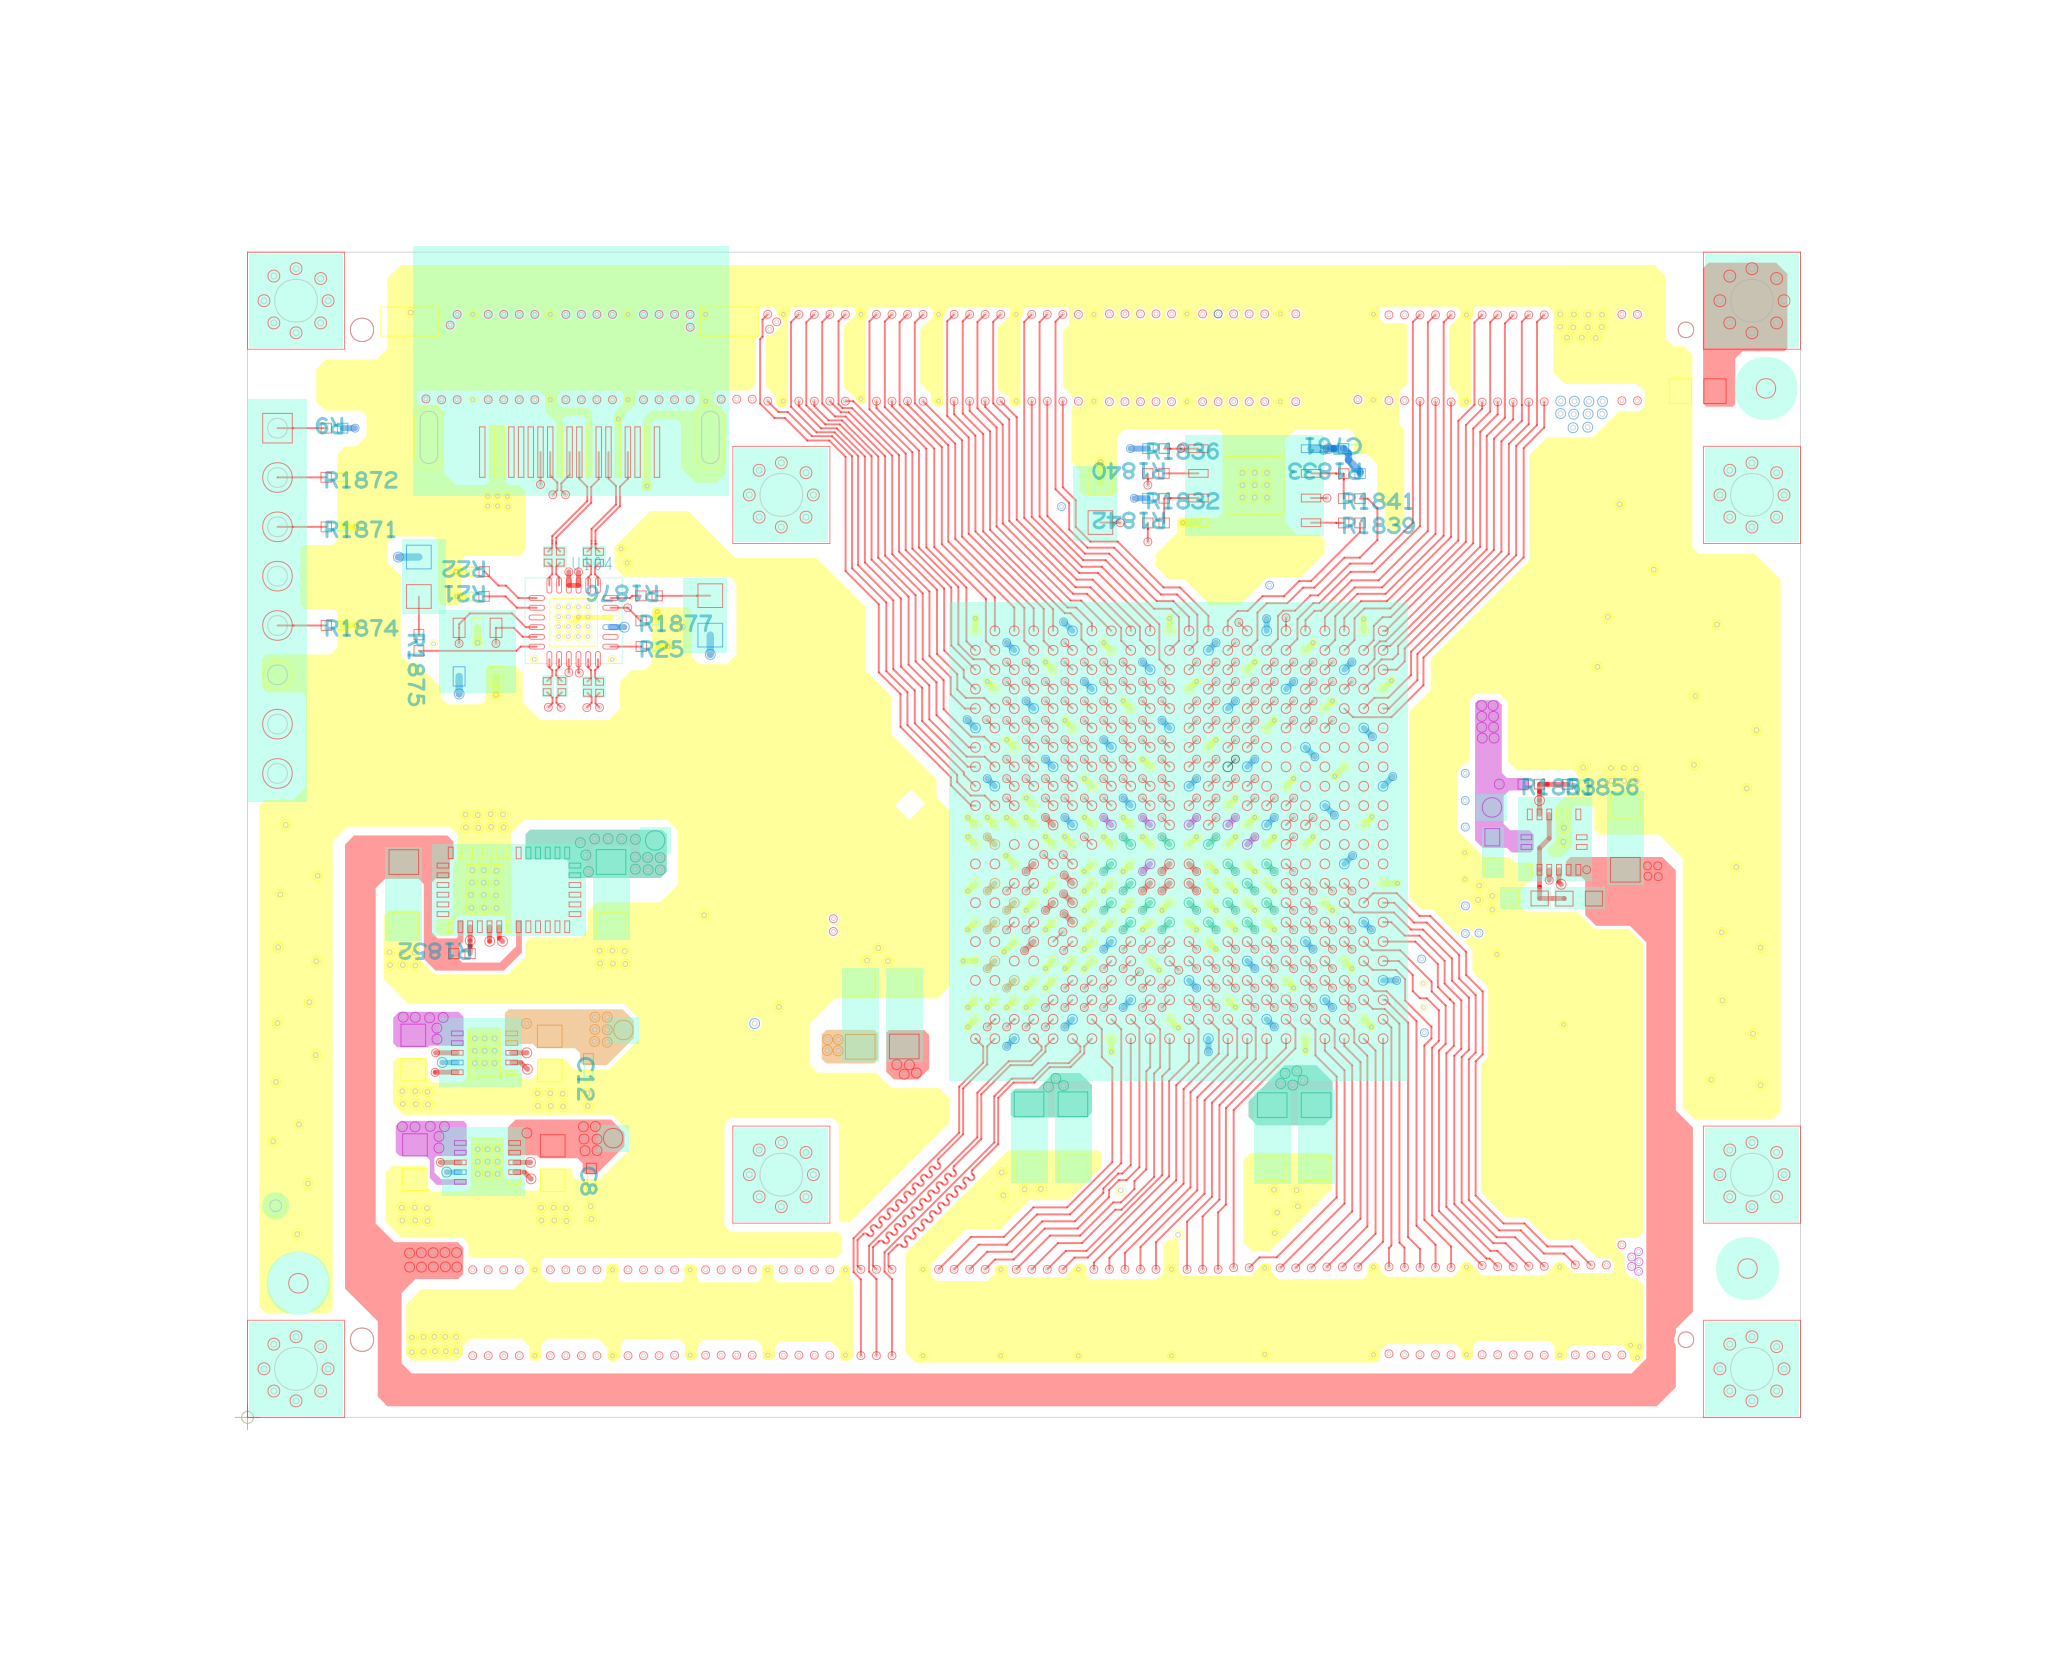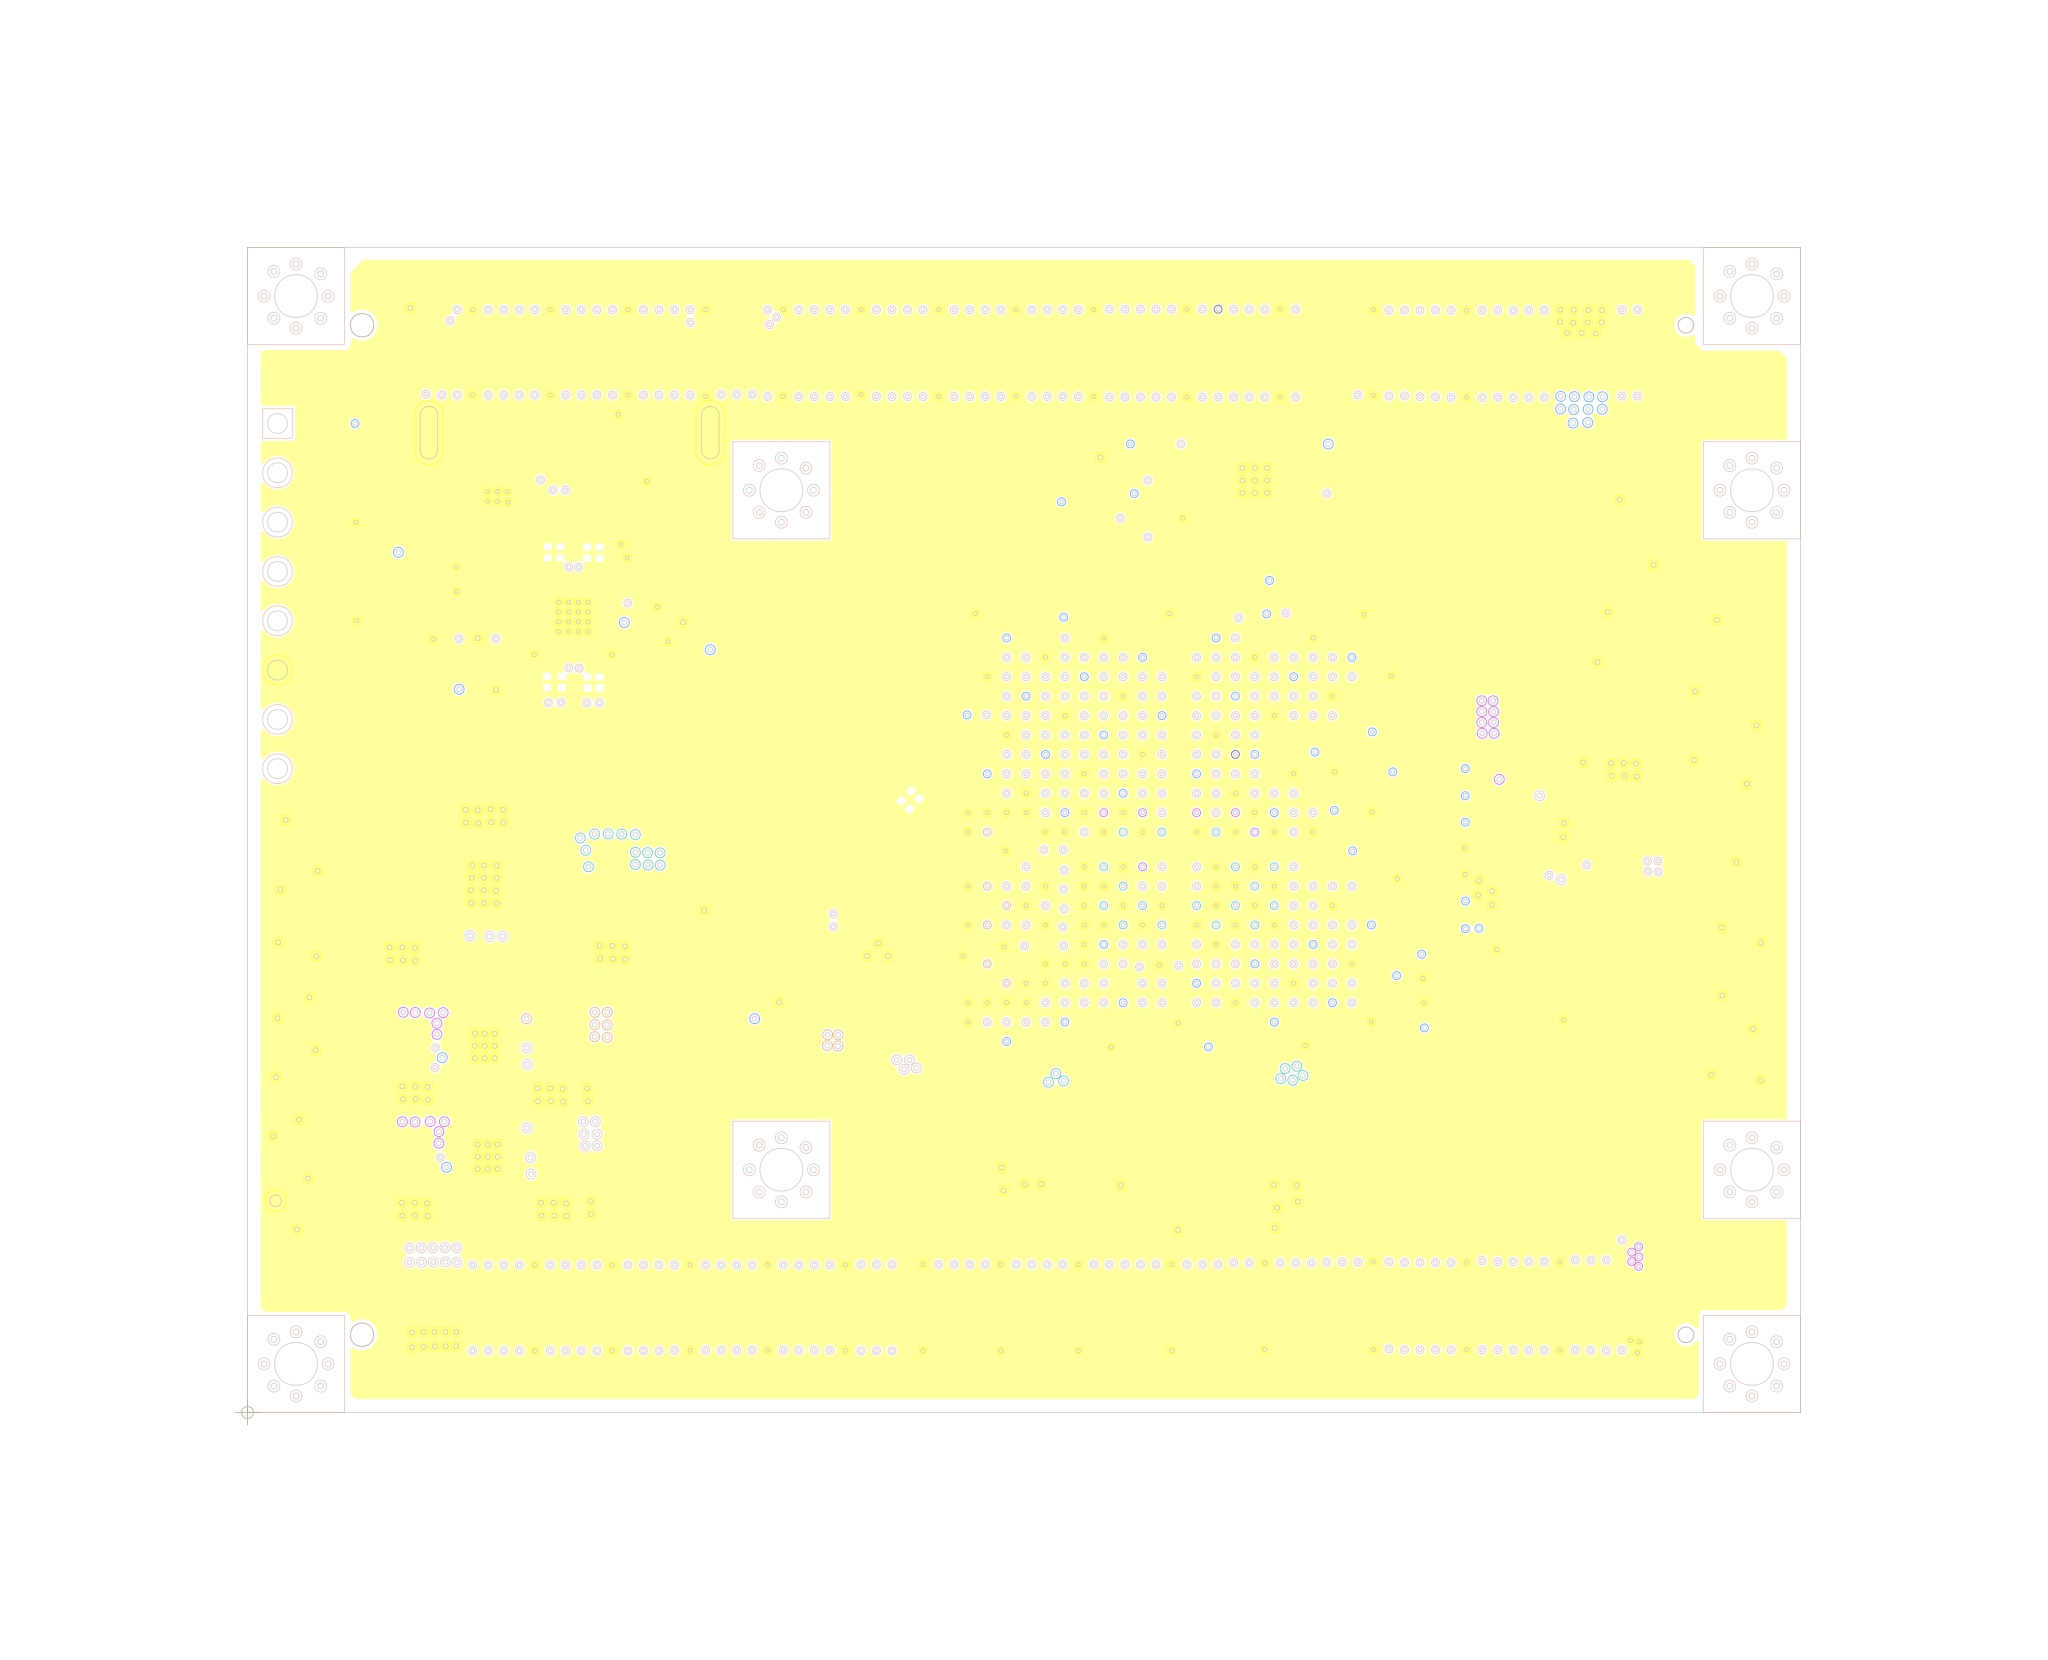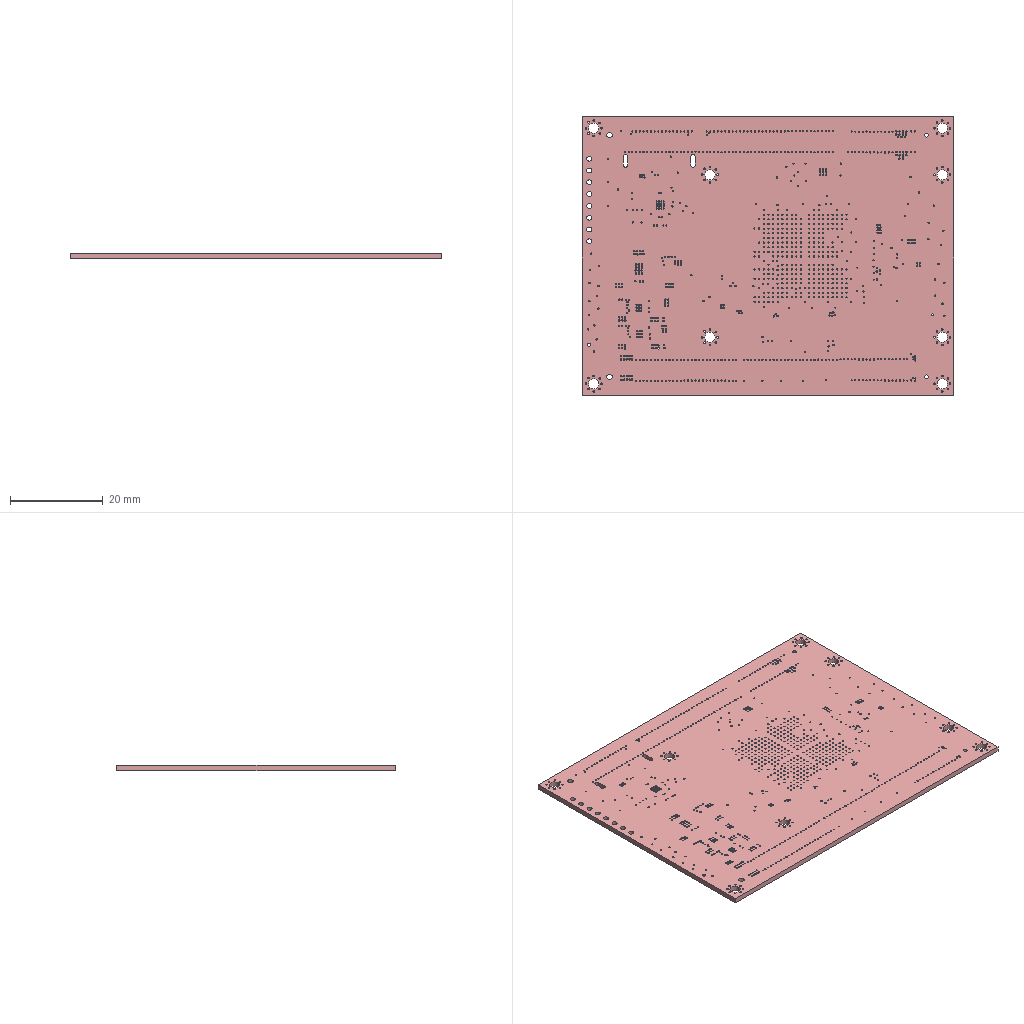Circuit board layout | Cadence Allegro | box 80 x 60 x 1.1 mm
Layer stack:
# Cadence Allegro layer stack of  (unit mm; from the constraint file cross-section; dielectric type: 0 not recorded (Allegro does not mark core vs prepreg), 3 surface material)
index,name,kind,layer,copper_thickness_mm,dielectric_type,dielectric_thickness_mm,dielectric_material,dielectric_constant
0,Top Surface,other,,,,,,
1,TOP,copper,TOP,0.0305,,,,
2,Dielectric1,dielectric,,,0,0.2032,FR-4,4.5
3,GND2,copper,GND2,0.0305,,,,
4,Dielectric2,dielectric,,,0,0.2032,FR-4,4.5
5,SIG3,copper,SIG3,0.0305,,,,
6,Dielectric3,dielectric,,,0,0.2032,FR-4,4.5
7,SIG4,copper,SIG4,0.0305,,,,
8,Dielectric4,dielectric,,,0,0.2032,FR-4,4.5
9,POWER5,copper,POWER5,0.0305,,,,
10,Dielectric5,dielectric,,,0,0.2032,FR-4,4.5
11,BOTTOM,copper,BOTTOM,0.0305,,,,
12,Bottom Surface,other,,,,,,
# drill layer pairs: low layer,high layer
drill_pair,TOP,BOTTOM
Part placement:
REFDES,COMP_VALUE,SYM_NAME,SYM_X,SYM_Y,SYM_ROTATE,SYM_MIRROR
C1,0.47uF/6.3V/10%/X5R/C0201,0201,1815.268,1086.576,180.000,YES
C2,0.47uF/6.3V/10%/X5R/C0201,0201,1815.260,1047.565,180.000,YES
C3,0.1uF/25V/10%/X5R/C0201,0201,1354.244,1251.889,135.000,YES
C4,0.1uF/25V/10%/X5R/C0201,0201,1334.672,1231.394,135.000,YES
C5,10uF/6.3V/10%/X5R/C0805,0805,339.614,517.452,270.000,NO
C6,0.1uF/50V/10%/X7R/C0402,0402,431.307,513.971,270.000,YES
C7,270P/6.3V/20%/X5R/C0402,0402,618.658,483.605,180.000,YES
C8,0.1uF/50V/10%/X7R/C0402,0402,697.516,488.137,270.000,NO
C9,47uF/6.3V/20%/X5R/C0805,0805,619.107,515.507,270.000,NO
C10,0.1uF/50V/10%/X7R/C0402,0402,425.205,736.184,270.000,YES
C11,47uF/6.3V/20%/X5R/C0805,0805,613.004,737.719,270.000,NO
C12,0.1uF/50V/10%/X7R/C0402,0402,691.414,710.349,270.000,NO
C13,10uF/6.3V/10%/X5R/C0805,0805,336.197,739.664,270.000,NO
C14,270P/6.3V/20%/X5R/C0402,0402,612.555,705.818,180.000,YES
C66,0.1uF/25V/10%/X5R/C0201,0201,2553.761,841.768,180.000,YES
C67,0.1uF/25V/10%/X5R/C0201,0201,2553.608,877.076,180.000,YES
C761,0.1uF/50V/10%/X7R/C0402,0402,2239.425,1964.287,180.000,NO
C763,100uF/6.3V/20%/X5R/C1206,T_1206,1773.209,569.491,90.000,YES
C764,4.7uF/6.3V/20%/X5R/C0402,0402,1887.404,1430.555,270.000,YES
C765,4.7uF/6.3V/20%/X5R/C0402,0402,2236.186,1189.759,180.000,YES
C766,100uF/6.3V/20%/X5R/C1206,T_1206,1585.041,570.750,270.000,NO
C767,100uF/6.3V/20%/X5R/C1206,T_1206,2119.165,569.587,90.000,YES
C768,100uF/6.3V/20%/X5R/C1206,T_1206,1673.984,570.757,270.000,NO
C769,0.47uF/6.3V/10%/X5R/C0201,0201,1925.198,1047.843,180.000,YES
C770,0.47uF/6.3V/10%/X5R/C0201,0201,2062.668,987.705,270.000,YES
C771,0.47uF/6.3V/10%/X5R/C0201,0201,1736.834,929.305,0.000,YES
C772,0.47uF/6.3V/10%/X5R/C0201,0201,1889.278,885.073,0.000,YES
C773,0.47uF/6.3V/10%/X5R/C0201,0201,1775.691,1236.027,180.000,YES
C774,0.47uF/6.3V/10%/X5R/C0201,0201,1559.332,791.280,270.000,YES
C775,0.47uF/6.3V/10%/X5R/C0201,0201,1983.760,989.024,270.000,YES
C776,0.47uF/6.3V/10%/X5R/C0201,0201,2101.346,1104.985,90.000,YES
C777,0.47uF/6.3V/10%/X5R/C0201,0201,2023.330,1028.285,90.000,YES
C778,0.47uF/6.3V/10%/X5R/C0201,0201,1756.062,1067.612,90.000,YES
C779,100uF/6.3V/20%/X5R/C1206,T_1206,1331.994,815.845,90.000,NO
C780,4.7uF/6.3V/20%/X5R/C0402,0402,1576.705,907.539,135.000,YES
C781,0.47uF/6.3V/10%/X5R/C0201,0201,1597.403,1008.921,0.000,YES
C782,100uF/6.3V/20%/X5R/C1206,T_1206,1379.805,1504.170,270.000,YES
C783,4.7uF/6.3V/20%/X5R/C0402,0402,1889.664,1311.894,270.000,YES
C784,4.7uF/6.3V/20%/X5R/C0402,0402,2264.650,1572.043,270.000,YES
C785,100uF/6.3V/20%/X5R/C1206,T_1206,2431.893,1489.047,270.000,YES
C786,4.7uF/6.3V/20%/X5R/C0402,0402,1890.236,1206.849,90.000,YES
C787,0.47uF/6.3V/10%/X5R/C0201,0201,2023.094,1215.693,90.000,YES
C788,0.47uF/6.3V/10%/X5R/C0201,0201,2063.562,1154.163,180.000,YES
C789,0.47uF/6.3V/10%/X5R/C0201,0201,1677.735,1215.385,90.000,YES
C790,0.47uF/6.3V/10%/X5R/C0201,0201,2102.239,1215.741,90.000,YES
C791,0.47uF/6.3V/10%/X5R/C0201,0201,1983.995,1413.098,90.000,YES
C792,0.47uF/6.3V/10%/X5R/C0201,0201,1776.037,1354.228,180.000,YES
C793,100uF/6.3V/20%/X5R/C1206,T_1206,1242.639,815.169,90.000,NO
C794,4.7uF/6.3V/20%/X5R/C0402,0402,1489.472,1027.803,0.000,YES
C795,0.47uF/6.3V/10%/X5R/C0201,0201,1483.481,934.388,0.000,YES
C796,100uF/6.3V/20%/X5R/C1206,T_1206,2167.176,569.035,270.000,NO
C797,4.7uF/6.3V/20%/X5R/C0402,0402,1887.876,983.961,90.000,YES
C798,100uF/6.3V/20%/X5R/C1206,T_1206,2078.175,569.035,270.000,NO
C799,4.7uF/6.3V/20%/X5R/C0402,0402,1757.832,1143.819,0.000,YES
C800,100uF/6.3V/20%/X5R/C1206,T_1206,2276.161,1387.556,270.000,YES
C801,4.7uF/6.3V/20%/X5R/C0402,0402,2083.622,1363.955,270.000,YES
C802,4.7uF/6.3V/20%/X5R/C0402,0402,2253.888,1026.907,0.000,YES
C803,0.47uF/6.3V/10%/X5R/C0201,0201,1795.243,988.367,90.000,YES
C804,0.47uF/6.3V/10%/X5R/C0201,0201,1716.691,1027.863,90.000,YES
C805,0.47uF/6.3V/10%/X5R/C0201,0201,1983.080,1153.632,180.000,YES
C806,0.47uF/6.3V/10%/X5R/C0201,0201,1834.935,1150.180,0.000,YES
C807,0.47uF/6.3V/10%/X5R/C0201,0201,2062.603,1066.526,270.000,YES
C808,0.47uF/6.3V/10%/X5R/C0201,0201,2229.205,801.348,180.000,YES
C809,0.47uF/6.3V/10%/X5R/C0201,0201,1795.599,1490.563,90.000,YES
C810,0.47uF/6.3V/10%/X5R/C0201,0201,1638.059,1373.665,270.000,YES
C811,0.47uF/6.3V/10%/X5R/C0201,0201,2003.454,929.020,0.000,YES
C812,100uF/6.3V/20%/X5R/C1206,T_1206,737.288,1061.971,270.000,NO
C813,22uF/10V/10%/X5R/C1206,T_1206,316.977,1061.767,270.000,NO
C814,22uF/10V/10%/X5R/C1206,T_1206,2794.433,1174.181,90.000,NO
C815,1uF/6.3V/10%/X5R/C0603,0603,2794.306,1140.592,270.000,YES
C816,22uF/6.3V/20%/X5R/C0603,0603,2524.563,1146.217,270.000,NO
C817,22pF/6.3V/5%/NP0/C0402,0402,620.211,992.251,0.000,YES
C818,5pF/25V/5%/NP0/C0402,0402,2603.653,1283.717,180.000,YES
C819,1uF/6.3V/10%/X5R/C0603,0603,2590.626,1052.032,0.000,NO
C820,47nF/6.3V/20%/X5R/C0402,0402,490.717,921.898,90.000,YES
C821,0.47uF/6.3V/10%/X5R/C0201,0201,2544.899,918.504,0.000,YES
C822,100uF/6.3V/20%/X5R/C1206,T_1206,1915.695,569.274,90.000,YES
C823,4.7uF/6.3V/20%/X5R/C0402,0402,1510.605,1589.385,270.000,YES
C824,4.7uF/6.3V/20%/X5R/C0402,0402,2191.766,1141.334,0.000,YES
C825,0.47uF/6.3V/10%/X5R/C0201,0201,1657.482,1511.176,0.000,YES
C826,0.47uF/6.3V/10%/X5R/C0201,0201,2200.327,929.252,180.000,YES
C827,0.47uF/6.3V/10%/X5R/C0201,0201,2161.046,1472.120,180.000,YES
C828,0.47uF/6.3V/10%/X5R/C0201,0201,1631.527,1602.546,90.000,YES
C829,100uF/6.3V/20%/X5R/C1206,T_1206,1878.663,1597.776,270.000,YES
C830,4.7uF/6.3V/20%/X5R/C0402,0402,2110.825,772.539,90.000,YES
C831,4.7uF/6.3V/20%/X5R/C0402,0402,1477.325,1457.153,270.000,YES
C832,0.47uF/6.3V/10%/X5R/C0201,0201,1518.712,1275.284,180.000,YES
C833,0.47uF/6.3V/10%/X5R/C0201,0201,1559.671,1412.480,90.000,YES
C834,0.47uF/6.3V/10%/X5R/C0201,0201,2299.640,885.476,0.000,YES
C835,0.47uF/6.3V/10%/X5R/C0201,0201,2165.367,1307.554,90.000,YES
C836,0.47uF/6.3V/10%/X5R/C0201,0201,2067.125,1582.210,90.000,YES
C837,0.47uF/6.3V/10%/X5R/C0201,0201,1938.895,1572.432,270.000,YES
C838,0.47uF/6.3V/10%/X5R/C0201,0201,2279.467,957.301,90.000,YES
C839,0.47uF/6.3V/10%/X5R/C0201,0201,1657.467,741.782,90.000,YES
C840,0.47uF/6.3V/10%/X5R/C0201,0201,2272.044,1508.412,180.000,YES
C841,0.1uF/25V/10%/X5R/C0201,0201,1091.785,1018.124,0.000,YES
C842,0.1uF/25V/10%/X5R/C0201,0201,1092.006,976.256,0.000,YES
C843,0.47uF/6.3V/10%/X5R/C0201,0201,1077.888,863.095,90.000,YES
C855,0.1u/50V/5%/X7R/C0402,0402,623.509,1686.667,0.000,YES
C856,0.1u/50V/5%/X7R/C0402,0402,704.621,1686.539,180.000,YES
C857,0.1u/50V/5%/X7R/C0402,0402,735.741,1618.439,270.000,YES
C858,10uF/6.3V/20%/X5R/C0603,0603,822.973,1602.371,180.000,YES
C859,0.1u/50V/5%/X7R/C0402,0402,377.293,1518.343,270.000,YES
C860,0.1uF/25V/10%/X5R/C0201,0201,607.625,1481.323,270.000,NO
C861,0.1uF/25V/10%/X5R/C0201,0201,637.597,1481.323,270.000,NO
C862,0.1uF/25V/10%/X5R/C0201,0201,634.433,1744.019,270.000,NO
C863,0.1uF/25V/10%/X5R/C0201,0201,609.649,1744.023,270.000,NO
C864,0.1uF/25V/10%/X5R/C0201,0201,689.329,1480.323,270.000,NO
C865,0.1uF/25V/10%/X5R/C0201,0201,713.965,1743.595,270.000,NO
C866,0.1uF/25V/10%/X5R/C0201,0201,714.117,1480.183,270.000,NO
C867,0.1uF/25V/10%/X5R/C0201,0201,689.181,1743.743,270.000,NO
D1,LED_RED,LED0805,347.573,1704.151,270.000,NO
D2,LED_RED,LED0805,938.565,1625.835,90.000,NO
D114,LED_GREEN,LED0805,1729.824,1854.068,90.000,NO
GND1,TEST POINT A,D0_6,57.041,429.175,270.000,NO
J2,HDMI,HDMI_A1,653.309,1956.903,180.000,NO
J42,Jumper 1K ohm,0402-3P,2105.937,1712.079,180.000,YES
J175,D2_3,D2_3,98.425,2263.780,270.000,NO
J176,D2_3,D2_3,98.425,98.425,270.000,NO
J177,D2_3,D2_3,3051.181,2263.780,270.000,NO
J178,D2_3,D2_3,3051.181,98.425,270.000,NO
J179,D2_3,D2_3,3051.181,1870.079,270.000,NO
J180,D2_3,D2_3,3051.181,492.126,270.000,NO
J181,D2_3,D2_3,1082.677,492.126,270.000,NO
J182,D2_3,D2_3,1082.677,1870.079,270.000,NO
J183,DIP-8_2_54mm,DIP8X1,60.789,1655.403,270.000,NO
JX1,5177983-8,5177984-8,1574.803,2204.724,0.000,YES
JX2,5177983-8,5177984-8,1574.803,157.480,0.000,YES
L1,BLM15AG100SN1,0402,1890.003,1117.234,270.000,YES
L2,BLM15AG100SN1,0402,2540.238,981.830,180.000,YES
L3,BLM15AG100SN1,0402,1028.502,857.588,270.000,YES
R3,4.7k/62.5mW/1%/R0402,0402,2428.842,1250.587,0.000,YES
R4,4.7k/62.5mW/1%/R0402,0402,2428.212,980.949,0.000,YES
R5,240R/62.5mW/1%/R0402,0402,1650.789,1797.504,90.000,YES
R6,4.7k/62.5mW/1%/R0402,0402,2428.559,1305.626,0.000,YES
R8,100R/62.5mW/1%/R0402,0402,1614.767,1109.446,135.000,YES
R9,1K/62.5mW/1%/R0402,0402,176.333,2005.411,180.000,NO
R10,10K/62.5mW/1%/R0402,0402,341.220,533.194,90.000,YES
R11,1K/62.5mW/1%/R0402,0402,542.512,560.149,90.000,YES
R12,3.9K/62.5mW/1%/R0402,0402,542.327,476.511,270.000,YES
R13,10K/62.5mW/1%/R0402,0402,340.637,755.981,90.000,YES
R14,2.49K/62.5mW/1%/R0402,0402,535.284,782.026,90.000,YES
R15,4.99K/62.5mW/1%/R0402,0402,535.240,698.176,270.000,YES
R16,1K/62.5mW/1%/R0402,0402,703.089,1536.307,180.000,YES
R17,4.7K/62.5mW/1%/R0402,0402,503.805,1518.343,270.000,YES
R19,4.7K/62.5mW/1%/R0402,0402,429.069,1518.595,270.000,YES
R20,1K/62.5mW/1%/R0402,0402,622.489,1536.815,0.000,YES
R21,1K/62.5mW/1%/R0402,0402,463.265,1664.455,180.000,NO
R22,1K/62.5mW/1%/R0402,0402,463.497,1714.779,180.000,NO
R25,1K/62.5mW/1%/R0402,0402,815.133,1562.811,0.000,NO
R79,10K/62.5mW/1%/R0402,0402,2652.769,982.070,0.000,YES
R1832,4.7k/62.5mW/1%/R0402,0402,1842.537,1863.279,0.000,NO
R1833,4.7k/62.5mW/1%/R0402,0402,2239.933,1913.267,180.000,NO
R1836,4.7k/62.5mW/1%/R0402,0402,1842.689,1963.985,0.000,NO
R1839,100R/62.5mW/1%/R0402,0402,2239.677,1813.279,0.000,NO
R1840,100R/62.5mW/1%/R0402,0402,1842.277,1913.779,180.000,NO
R1841,100R/62.5mW/1%/R0402,0402,2239.677,1862.511,0.000,NO
R1842,100R/62.5mW/1%/R0402,0402,1842.537,1813.287,180.000,NO
R1845,1K/62.5mW/1%/R0402/NI,0402,2428.110,1037.039,0.000,YES
R1846,100R/62.5mW/1%/R0402,0402,1718.069,1797.221,90.000,YES
R1847,1K/62.5mW/1%/R0402,0402,2428.905,1196.799,0.000,YES
R1848,1K/62.5mW/1%/R0402,0402,2428.279,1144.740,180.000,YES
R1849,1K/62.5mW/1%/R0402,0402,2428.098,1091.134,180.000,YES
R1851,100K/62.5mW/1%/R0402,0402,2657.059,1110.327,180.000,YES
R1852,200K/62.5mW/1%/R0402,0402,434.988,940.132,180.000,NO
R1853,237K/62.5mW/1%/R0402,0402,2603.775,1283.563,0.000,NO
R1854,200K/62.5mW/1%/R0402,0402,620.013,938.572,0.000,YES
R1855,10R/100mW/1%/R0603,0603,2700.787,1051.689,0.000,NO
R1856,118K/62.5mW/1%/R0402,0402,2693.673,1283.256,0.000,NO
R1857,604K/62.5mW/1%/R0402,0402,540.726,921.960,270.000,YES
R1859,0R/125mW/1%/R0805,0805,2941.194,2080.455,180.000,NO
R1860,130R/62.5mW/1%/R0402,0402,2428.687,779.874,180.000,YES
R1861,130R/62.5mW/1%/R0402,0402,2428.315,929.230,180.000,YES
R1862,100R/62.5mW/1%/R0402,0402,2503.505,859.296,270.000,YES
R1863,82R/62.5mW/1%/R0402,0402,2428.883,830.958,0.000,YES
R1864,82R/62.5mW/1%/R0402,0402,2428.063,879.942,0.000,YES
R1865,10K/62.5mW/1%/R0402,0402,964.894,858.389,90.000,YES
R1866,100R/62.5mW/1%/R0402,0402,1153.606,997.399,270.000,YES
R1871,20K/62.5mW/1%/R0402,0402,176.241,1805.343,0.000,NO
R1872,1K/62.5mW/1%/R0402 NI**,0402,175.885,1905.675,0.000,NO
R1874,1K/62.5mW/1%/R0402,0402,176.333,1605.399,0.000,NO
R1875,4.7K/62.5mW/1%/R0402,0402,347.573,1570.495,270.000,NO
R1876,4.7K/62.5mW/1%/R0402,0402,814.317,1665.511,180.000,NO
R1877,1K/62.5mW/1%/R0402,0402,814.597,1614.819,0.000,NO
TP85,TEST POINT A,TEST_12MM,826.710,1169.585,0.000,NO
TP86,TEST POINT A,TEST_12MM,2523.881,1236.553,180.000,NO
TP87,TEST POINT A,TEST_12MM,741.578,566.118,0.000,NO
TP88,TEST POINT A,TEST_12MM,762.391,785.339,0.000,NO
TP89,TEST POINT A,TEST_12MM,2500.805,793.503,0.000,YES
TP90,TEST POINT A,TEST_12MM,2501.702,922.799,0.000,YES
TP91,TEST POINT A,TEST_12MM,1102.797,1061.449,180.000,YES
TP92,TEST POINT A,TEST_12MM,1103.608,931.449,180.000,YES
U1,xc7a35tfgg484,FGG484_23X23,1889.764,1181.102,90.000,NO
U2,TPS74801DRCR,VSON-10,486.677,516.932,0.000,NO
U4,TPS74801DRCR,VSON-10,480.575,739.145,0.000,NO
U100,MT25QL128ABA1EW7,WPDFN-8_6X5,2042.761,1888.779,0.000,NO
U102,EN6347QI,EN6347QI,530.236,1069.483,180.000,NO
U103,EP53F8QI,QFN-16_3X3,2649.846,1166.276,270.000,NO
U104,DS80PCI102SQE/NOPB,QFN-24_4X4_1,661.471,1611.841,0.000,NO
U105,AT24C01C-STUM-T,SOT_23_5,466.609,1551.399,0.000,NO
X2,DSC1122CI2-125,VDFN-3225,2637.806,877.176,0.000,YES
X3,DSC1122CI2-125,VDFN-3225,997.100,976.688,180.000,YES
Pad and via stacks, first 117 of 273 lines:
# Allegro (Cadence) via spans and padstacks; design units: ("mils" 3 1000)
# via spans: padstack,start_layer,end_layer,net_example,count
VIA1020,ETCH/TOP,ETCH/BOTTOM,GND,272
VIA8-BGA-Q,ETCH/TOP,ETCH/BOTTOM,GND,704
# Allegro padstack definitions: name,start_layer,end_layer,drill,plating,holeType,type
PAD19,"ETCH/TOP","ETCH/TOP",0.0,"NON_PLATED","none","smd"
PAD13,"ETCH/TOP","ETCH/TOP",0.0,"NON_PLATED","none","smd"
PAD12,"ETCH/TOP","ETCH/TOP",0.0,"NON_PLATED","none","smd"
PAD17,"ETCH/TOP","ETCH/TOP",0.0,"NON_PLATED","none","smd"
PAD15,"ETCH/TOP","ETCH/TOP",0.0,"NON_PLATED","none","smd"
PAD16,"ETCH/TOP","ETCH/TOP",0.0,"NON_PLATED","none","smd"
PAD1,"ETCH/TOP","ETCH/TOP",0.0,"NON_PLATED","none","smd"
PAD46,"ETCH/TOP","ETCH/TOP",0.0,"NON_PLATED","none","smd"
PAD44,"ETCH/TOP","ETCH/TOP",0.0,"NON_PLATED","none","smd"
PAD8,"ETCH/TOP","ETCH/TOP",0.0,"NON_PLATED","none","smd"
PAD5,"ETCH/TOP","ETCH/TOP",0.0,"NON_PLATED","none","smd"
PAD9,"ETCH/TOP","ETCH/TOP",0.0,"NON_PLATED","none","smd"
PAD10,"ETCH/TOP","ETCH/TOP",0.0,"NON_PLATED","none","smd"
PAD25,"ETCH/TOP","ETCH/TOP",0.0,"NON_PLATED","none","smd"
PAD4,"ETCH/TOP","ETCH/TOP",0.0,"NON_PLATED","none","smd"
PAD7,"ETCH/TOP","ETCH/TOP",0.0,"NON_PLATED","none","smd"
PAD6,"ETCH/TOP","ETCH/TOP",0.0,"NON_PLATED","none","smd"
PAD3,"ETCH/TOP","ETCH/TOP",0.0,"NON_PLATED","none","smd"
PAD31,"ETCH/TOP","ETCH/TOP",0.0,"NON_PLATED","none","smd"
PAD22,"ETCH/TOP","ETCH/TOP",0.0,"NON_PLATED","none","smd"
PAD41,"ETCH/TOP","ETCH/TOP",0.0,"NON_PLATED","none","smd"
PAD42,"ETCH/TOP","ETCH/TOP",0.0,"NON_PLATED","none","smd"
PAD43,"ETCH/TOP","ETCH/TOP",0.0,"NON_PLATED","none","smd"
PAD45,"ETCH/TOP","ETCH/TOP",0.0,"NON_PLATED","none","smd"
PAD2,"ETCH/TOP","ETCH/TOP",0.0,"NON_PLATED","none","smd"
PAD14,"ETCH/TOP","ETCH/TOP",0.0,"NON_PLATED","none","smd"
PAD21,"ETCH/TOP","ETCH/TOP",0.0,"NON_PLATED","none","smd"
PAD28,"ETCH/TOP","ETCH/TOP",0.0,"NON_PLATED","none","smd"
PAD26,"ETCH/TOP","ETCH/TOP",0.0,"NON_PLATED","none","smd"
PAD27,"ETCH/TOP","ETCH/TOP",0.0,"NON_PLATED","none","smd"
PAD18,"ETCH/TOP","ETCH/TOP",0.0,"NON_PLATED","none","smd"
PAD29,"ETCH/TOP","ETCH/TOP",0.0,"NON_PLATED","none","smd"
PAD20,"ETCH/TOP","ETCH/TOP",0.0,"NON_PLATED","none","smd"
PAD39,"ETCH/TOP","ETCH/TOP",0.0,"NON_PLATED","none","smd"
PAD40,"ETCH/TOP","ETCH/TOP",0.0,"NON_PLATED","none","smd"
PAD30,"ETCH/TOP","ETCH/TOP",0.0,"NON_PLATED","none","smd"
PAD48,"ETCH/TOP","ETCH/TOP",0.0,"NON_PLATED","none","smd"
PAD47,"ETCH/TOP","ETCH/TOP",0.0,"NON_PLATED","none","smd"
PAD49,"ETCH/TOP","ETCH/TOP",0.0,"NON_PLATED","none","smd"
PAD50,"ETCH/TOP","ETCH/TOP",0.0,"NON_PLATED","none","smd"
PAD53,"ETCH/TOP","ETCH/TOP",0.0,"NON_PLATED","none","smd"
F45,"ETCH/TOP","ETCH/TOP",0.0,"NON_PLATED","none","smd"
R88X76,"ETCH/TOP","ETCH/TOP",0.0,"PLATED","none","smd"
R127X121,"ETCH/TOP","ETCH/TOP",0.0,"PLATED","none","smd"
R14X25,"ETCH/TOP","ETCH/TOP",0.0,"NON_PLATED","none","smd"
R165X317,"ETCH/TOP","ETCH/TOP",0.0,"NON_PLATED","none","smd"
R259X218,"ETCH/TOP","ETCH/TOP",0.0,"NON_PLATED","none","smd"
R70X22,"ETCH/TOP","ETCH/TOP",0.0,"NON_PLATED","none","smd"
R75X85,"ETCH/TOP","ETCH/TOP",0.0,"NON_PLATED","none","smd"
Y5,"ETCH/TOP","ETCH/TOP",0.0,"NON_PLATED","none","smd"
R16X30,"ETCH/TOP","ETCH/TOP",0.0,"NON_PLATED","none","smd"
F62X58,"ETCH/TOP","ETCH/TOP",0.0,"NON_PLATED","none","smd"
R15X28,"ETCH/TOP","ETCH/TOP",0.0,"NON_PLATED","none","smd"
R195X280,"ETCH/TOP","ETCH/TOP",0.0,"NON_PLATED","none","smd"
R45X200,"ETCH/TOP","ETCH/TOP",0.0,"NON_PLATED","none","smd"
R50X30,"ETCH/TOP","ETCH/TOP",0.0,"NON_PLATED","none","smd"
R127X120,"ETCH/TOP","ETCH/TOP",0.0,"PLATED","none","smd"
R31X24,"ETCH/TOP","ETCH/TOP",0.0,"NON_PLATED","none","smd"
R215X60,"ETCH/TOP","ETCH/TOP",0.0,"NON_PLATED","none","smd"
S17,"ETCH/TOP","ETCH/TOP",0.0,"NON_PLATED","none","smd"
R23X25,"ETCH/TOP","ETCH/TOP",0.0,"NON_PLATED","none","smd"
R19X32,"ETCH/TOP","ETCH/TOP",0.0,"NON_PLATED","none","smd"
R61X15,"ETCH/TOP","ETCH/TOP",0.0,"NON_PLATED","none","smd"
R45X150,"ETCH/TOP","ETCH/TOP",0.0,"NON_PLATED","none","smd"
R12X8,"ETCH/TOP","ETCH/TOP",0.0,"NON_PLATED","none","smd"
R91X127,"ETCH/TOP","ETCH/TOP",0.0,"PLATED","none","smd"
S91,"ETCH/TOP","ETCH/TOP",0.0,"PLATED","none","smd"
R55X99,"ETCH/TOP","ETCH/TOP",0.0,"NON_PLATED","none","smd"
R299X199,"ETCH/TOP","ETCH/TOP",0.0,"NON_PLATED","none","smd"
R114X165,"ETCH/TOP","ETCH/TOP",0.0,"NON_PLATED","none","smd"
R60X90,"ETCH/TOP","ETCH/TOP",0.0,"NON_PLATED","none","smd"
R6X10,"ETCH/TOP","ETCH/TOP",0.0,"NON_PLATED","none","smd"
Y10,"ETCH/TOP","ETCH/TOP",0.0,"PLATED","none","smd"
R114X74,"ETCH/TOP","ETCH/TOP",0.0,"NON_PLATED","none","smd"
R30X130,"ETCH/TOP","ETCH/TOP",0.0,"NON_PLATED","none","smd"
R50X127,"ETCH/TOP","ETCH/TOP",0.0,"NON_PLATED","none","smd"
R18X20,"ETCH/TOP","ETCH/TOP",0.0,"NON_PLATED","none","smd"
R60X71,"ETCH/TOP","ETCH/TOP",0.0,"NON_PLATED","none","smd"
R48X71,"ETCH/TOP","ETCH/TOP",0.0,"NON_PLATED","none","smd"
R80X30,"ETCH/TOP","ETCH/TOP",0.0,"PLATED","none","smd"
FLASH_0,"ETCH/TOP","ETCH/TOP",0.0,"PLATED","none","smd"
Y3,"ETCH/TOP","ETCH/TOP",0.0,"PLATED","none","smd"
R170X25,"ETCH/TOP","ETCH/TOP",0.0,"PLATED","none","smd"
R70X25,"ETCH/TOP","ETCH/TOP",0.0,"PLATED","none","smd"
R43X14,"ETCH/TOP","ETCH/TOP",0.0,"PLATED","none","smd"
R33X10,"ETCH/TOP","ETCH/TOP",0.0,"PLATED","none","smd"
R636X23,"ETCH/TOP","ETCH/TOP",0.0,"PLATED","none","smd"
R155X35,"ETCH/TOP","ETCH/TOP",0.0,"PLATED","none","smd"
R60X20,"ETCH/TOP","ETCH/TOP",0.0,"PLATED","none","smd"
R120X70,"ETCH/TOP","ETCH/TOP",0.0,"PLATED","none","smd"
SMD0_45R,"ETCH/TOP","ETCH/TOP",0.0,"PLATED","none","smd"
Y42,"ETCH/TOP","ETCH/TOP",0.0,"PLATED","none","smd"
R85X65,"ETCH/TOP","ETCH/TOP",0.0,"PLATED","none","smd"
Y30,"ETCH/TOP","ETCH/TOP",0.0,"PLATED","none","smd"
R53X20,"ETCH/TOP","ETCH/TOP",0.0,"PLATED","none","smd"
R55X40,"ETCH/TOP","ETCH/TOP",0.0,"PLATED","none","smd"
R155X25,"ETCH/TOP","ETCH/TOP",0.0,"PLATED","none","smd"
F17X17,"ETCH/TOP","ETCH/TOP",0.0,"PLATED","none","smd"
F89X32,"ETCH/TOP","ETCH/TOP",0.0,"PLATED","none","smd"
R8X2,"ETCH/TOP","ETCH/TOP",0.0,"PLATED","none","smd"
SMD40X20,"ETCH/TOP","ETCH/TOP",0.0,"PLATED","none","smd"
R340X185,"ETCH/TOP","ETCH/TOP",0.0,"PLATED","none","smd"
R27X10,"ETCH/TOP","ETCH/TOP",0.0,"PLATED","none","smd"
R22X11,"ETCH/TOP","ETCH/TOP",0.0,"PLATED","none","smd"
R32X36,"ETCH/TOP","ETCH/TOP",0.0,"PLATED","none","smd"
S21X20,"ETCH/TOP","ETCH/TOP",0.0,"PLATED","none","smd"
R13X10,"ETCH/TOP","ETCH/TOP",0.0,"PLATED","none","smd"
R75X28,"ETCH/TOP","ETCH/TOP",0.0,"PLATED","none","smd"
R25X15,"ETCH/TOP","ETCH/TOP",0.0,"NON_PLATED","none","smd"
C0_5,"ETCH/TOP","ETCH/TOP",0.0,"PLATED","none","smd"
S437,"ETCH/TOP","ETCH/TOP",0.0,"PLATED","none","smd"
R150X30,"ETCH/TOP","ETCH/TOP",0.0,"PLATED","none","smd"
Design rules, without the lines most boards share, first 19 of 44 lines:
# Cadence Allegro design rules of  (from the Constraint Manager export constraints.dcfx, design unit mil; typed fields in mm)
# columns: name | kind | enabled | priority | scope1 | scope2 | descriptor | typed fields (field=value)
# Allegro precedence (priority 1 wins): 1 Region class-to-class, 2 Region class, 3 Region, 4 class-to-class, 5 DiffPair/Bus/NetGroup override, 6 NetClass, 7 constraint set (CSet) default
# per-layer values are written LAYER=value in the descriptor and LAYER:mm in the typed field; a maximum of 0 means no limit set
# --- net classes (and buses / net groups) ---
PCIE_TX | NetClass | enabled | 6 | DIFFPAIR9, DIFFPAIR10, DIFFPAIR11, DIFFPAIR12 | All | Net Class (members: 4 DiffPair) overrides: (DIFFP_PHASE_TOL=5 mil) |  diffp_phase_tol=5mil
PCIE_RX | NetClass | enabled | 6 | DIFFPAIR5, DIFFPAIR6, DIFFPAIR7, DIFFPAIR8 | All | Net Class (members: 4 DiffPair) overrides: (DIFFP_PHASE_TOL=5 mil) |  diffp_phase_tol=5mil
# --- track widths, neck and differential-pair gap (physical constraint sets) ---
DEFAULT | PhysicalCSet | enabled | 7 | Design default | All | Physical Constraint (Min Line Width=4mil) (Max Line Width=0mil) (Min Neck Width=0mil) (Max Neck Length=0mil) (DiffPair Primary Gap=4mil) (DiffPair Neck Gap=0mil) (DiffPair Min Space=0mil) (DiffPair Coupled +Tol=0mil) (DiffPair Coupled -Tol=0mil) (Min BB Via Stagger=5mil) (Max BB Via Stagger=0mil) (T-junctions=ANYWHERE) (Pad-pad direct connect=ALL_ALLOWED) (Allowed vias=VIA8-BGA-Q, STANDARDVIA, POWERVIA, VIA1020) | min_line_width=0.1016 min_neck_width=0 min_bvia_stagger=0.127 max_bvia_stagger=0 ts_allowed=ANYWHERE diffp_primary_gap=0.1016 diffp_neck_gap=0 max_line_width=0 maximum_neck_length=0 pad_pad_direct_connect=ALL_ALLOWED allow_on_etch_subclass=TRUE diffp_coupled_plus=0 diffp_coupled_minus=0 diffp_min_space=0 vias=VIA8-BGA-Q,STANDARDVIA,POWERVIA,VIA1020
# --- clearances: line / pad / via / shape / hole (spacing constraint sets) ---
DEFAULT | SpacingCSet | enabled | 7 | Design default | All | Clearance Constraint (Line-Line=4mil) (Line-SMD Pad=TOP=4mil GND2=4mil SIG3=4mil SIG4=4mil POWER5=4mil BOTTOM=3.9mil) (Line-Thru Pin=4mil) (Line-Via=4mil) (Line-Shape=4mil) (SMD Pad-SMD Pad=4mil) (Thru Pin-Thru Pin=4mil) (Thru Pin-SMD Pad=4mil) (SMD Pad-Via=4mil) (Thru Pin-Via=4mil) (Via-Via=4mil) (Shape-SMD Pad=5mil) (Shape-Thru Pin=4mil) (Shape-Via=4mil) (Shape-Shape=6mil) (Hole-Hole=6mil) (Hole-Line=5mil) (Hole-Shape=10mil) (BB Via-BB Via=6mil) (uVia-uVia=6mil) | thrupin_to_thrupin_spacing=0.1016 thrupin_to_smdpin_spacing=0.1016 thrupin_to_thruvia_spacing=0.1016 line_to_thrupin_spacing=0.1016 thrupin_to_shape_spacing=0.1016 smdpin_to_smdpin_spacing=0.1016 smdpin_to_thruvia_spacing=0.1016 line_to_smdpin_spacing=TOP:0.1016,GND2:0.1016,SIG3:0.1016,SIG4:0.1016,POWER5:0.1016,BOTTOM:0.0991 shape_to_smdpin_spacing=0.127 thruvia_to_thruvia_spacing=0.1016 line_to_thruvia_spacing=0.1016 shape_to_thruvia_spacing=0.1016 line_to_line_spacing=0.1016 line_to_shape_spacing=0.1016 shape_to_shape_spacing=0.1524 bbv_to_bbv_spacing=0.1524 bbv_to_thrupin_spacing=0.1016 bbv_to_smdpin_spacing=0.127 bbv_to_thruvia_spacing=0.1016 bbv_to_line_spacing=0.127 bbv_to_shape_spacing=0.1524 bbv_to_testpin_spacing=0.127 bbv_to_testvia_spacing=0 testpin_to_testpin_spacing=0.127 testpin_to_thrupin_spacing=0.1016 smdpin_to_testpin_spacing=0.1016 testpin_to_thruvia_spacing=0.1016 testpin_to_testvia_spacing=0.127 line_to_testpin_spacing=0.1016 shape_to_testpin_spacing=0.127 testvia_to_testvia_spacing=0 testvia_to_thrupin_spacing=0.1016 smdpin_to_testvia_spacing=0.127 testvia_to_thruvia_spacing=0.1016 line_to_testvia_spacing=0.1016 shape_to_testvia_spacing=0.1524 bondpad_to_bondpad_spacing=0 thrupin_to_bondpad_spacing=0.1016 smdpin_to_bondpad_spacing=0.127 bondpad_to_thruvia_spacing=0.1016 bondpad_to_line_spacing=0.1016 bondpad_to_shape_spacing=0.1524 bondpad_to_bbv_spacing=0.1524 bondpad_to_testpin_spacing=0.127 bondpad_to_testvia_spacing=0.127 hole_to_pin_spacing=0.127 hole_to_via_spacing=0.1524 hole_to_line_spacing=0.127 hole_to_shape_spacing=0.254 hole_to_hole_spacing=0.1524 mvia_to_mvia_spacing=0.1524 mvia_to_thrupin_spacing=0.1016 mvia_to_smdpin_spacing=0.127 mvia_to_thruvia_spacing=0.1016 mvia_to_bbv_spacing=0.1524 mvia_to_line_spacing=0.1016 mvia_to_shape_spacing=0.1524 mvia_to_testpin_spacing=0.127 mvia_to_testvia_spacing=0.127 bondpad_to_mvia_spacing=0.127 bondpad_to_bondpad_diffp_spc=0.127 min_bvia_gap=0.127
DEFAULT | SameNetSpacingCSet | disabled (SAME_NET=FALSE) | 7 | Design default | All | Same-Net Clearance (Line-Line=0mil) (Line-SMD Pad=0mil) (Line-Thru Pin=0mil) (Line-Via=0mil) (Line-Shape=0mil) (SMD Pad-SMD Pad=0mil) (Thru Pin-Thru Pin=0mil) (Thru Pin-SMD Pad=0mil) (SMD Pad-Via=6mil) (Thru Pin-Via=0mil) (Via-Via=6mil) (Shape-SMD Pad=7.874mil) (Shape-Thru Pin=0mil) (Shape-Via=0mil) (Shape-Shape=0mil) (Hole-Hole=8mil) (Hole-Line=8mil) (Hole-Shape=8mil) (BB Via-BB Via=6mil) (uVia-uVia=6mil) | sn_thrupin_to_thrupin_spacing=0 sn_thrupin_to_smdpin_spacing=0 sn_thrupin_to_thruvia_spacing=0 sn_line_to_thrupin_spacing=0 sn_thrupin_to_shape_spacing=0 sn_smdpin_to_smdpin_spacing=0 sn_smdpin_to_thruvia_spacing=0.1524 sn_line_to_smdpin_spacing=0 sn_shape_to_smdpin_spacing=0.2 sn_thruvia_to_thruvia_spacing=0.1524 sn_line_to_thruvia_spacing=0 sn_shape_to_thruvia_spacing=0 sn_line_to_line_spacing=0 sn_line_to_shape_spacing=0 sn_shape_to_shape_spacing=0 sn_bbv_to_bbv_spacing=0.1524 sn_bbv_to_thrupin_spacing=0 sn_bbv_to_smdpin_spacing=0.1524 sn_bbv_to_thruvia_spacing=0.1524 sn_bbv_to_line_spacing=0 sn_bbv_to_shape_spacing=0 sn_bbv_to_testpin_spacing=0 sn_bbv_to_testvia_spacing=0 sn_testpin_to_testpin_spacing=0 sn_testpin_to_thrupin_spacing=0 sn_smdpin_to_testpin_spacing=0 sn_testpin_to_thruvia_spacing=0 sn_testpin_to_testvia_spacing=0 sn_line_to_testpin_spacing=0 sn_shape_to_testpin_spacing=0 sn_testvia_to_testvia_spacing=0 sn_testvia_to_thrupin_spacing=0 sn_smdpin_to_testvia_spacing=0 sn_testvia_to_thruvia_spacing=0 sn_line_to_testvia_spacing=0 sn_shape_to_testvia_spacing=0 sn_bondpad_to_bondpad_spacing=0 sn_thrupin_to_bondpad_spacing=0 sn_smdpin_to_bondpad_spacing=0 sn_bondpad_to_thruvia_spacing=0 sn_bondpad_to_line_spacing=0 sn_bondpad_to_shape_spacing=0 sn_bondpad_to_bbv_spacing=0.127 sn_bondpad_to_testpin_spacing=0.127 sn_bondpad_to_testvia_spacing=0.127 same_net=FALSE sn_hole_to_pin_spacing=0.2032 sn_hole_to_via_spacing=0.2032 sn_hole_to_line_spacing=0.2032 sn_hole_to_shape_spacing=0.2032 sn_hole_to_hole_spacing=0.2032 sn_mvia_to_mvia_spacing=0.1524 sn_mvia_to_thrupin_spacing=0.127 sn_mvia_to_smdpin_spacing=0.1524 sn_mvia_to_thruvia_spacing=0.1524 sn_mvia_to_bbv_spacing=0.1524 sn_mvia_to_line_spacing=0.127 sn_mvia_to_shape_spacing=0.127 sn_mvia_to_testpin_spacing=0.127 sn_mvia_to_testvia_spacing=0.127 sn_bondpad_to_mvia_spacing=0.127
# --- differential pairs (17) ---
DIFFPAIR9 | DiffPair | enabled | 5 | PCIE_TX0_N | PCIE_TX0_P | Differential Pair (Primary Gap=4mil) (Min Line Width=4mil) (Physical CSet=DEFAULT) | gap=0.1016 width=0.1016
DIFFPAIR10 | DiffPair | enabled | 5 | PCIE_TX1_N | PCIE_TX1_P | Differential Pair (Primary Gap=4mil) (Min Line Width=4mil) (Physical CSet=DEFAULT) | gap=0.1016 width=0.1016
DIFFPAIR11 | DiffPair | enabled | 5 | PCIE_TX2_N | PCIE_TX2_P | Differential Pair (Primary Gap=4mil) (Min Line Width=4mil) (Physical CSet=DEFAULT) | gap=0.1016 width=0.1016
DIFFPAIR12 | DiffPair | enabled | 5 | PCIE_TX3_N | PCIE_TX3_P | Differential Pair (Primary Gap=4mil) (Min Line Width=4mil) (Physical CSet=DEFAULT) | gap=0.1016 width=0.1016
DIFFPAIR5 | DiffPair | enabled | 5 | PCIE_RX0_N | PCIE_RX0_P | Differential Pair (Primary Gap=4mil) (Min Line Width=4mil) (Physical CSet=DEFAULT) overrides: (DIFFP_PHASE_TOL=2.5 mil) | gap=0.1016 width=0.1016  diffp_phase_tol=2.5mil
DIFFPAIR6 | DiffPair | enabled | 5 | PCIE_RX1_N | PCIE_RX1_P | Differential Pair (Primary Gap=4mil) (Min Line Width=4mil) (Physical CSet=DEFAULT) | gap=0.1016 width=0.1016